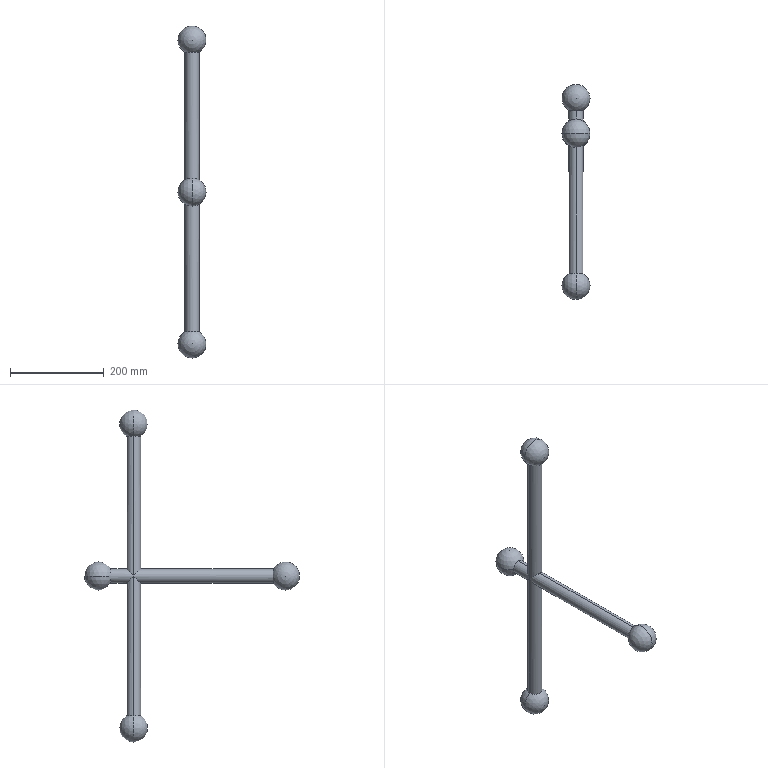Part | SolidWorks | features Revolution 3, ICE 2, Extrusion 1, MirrorPattern 1 | 1 solid | 16 faces | box 60 x 460 x 710 mm | volume 1097313 mm3 | sphere 8 | cylinder 8 | commonest cylinder face diameters 30 x8
STEP:
#1=CARTESIAN_POINT('',(0.,-355.,0.));
#2=VERTEX_POINT('',#1);
#3=CARTESIAN_POINT('',(0.,-299.019,-15.));
#4=VERTEX_POINT('',#3);
#5=CARTESIAN_POINT('',(0.,-325.,0.));
#6=DIRECTION('',(1.,0.,0.));
#7=DIRECTION('',(0.,0.,-1.));
#8=AXIS2_PLACEMENT_3D('',#5,#6,#7);
#9=CIRCLE('',#8,30.);
#10=EDGE_CURVE('',#2,#4,#9,.T.);
#11=ORIENTED_EDGE('',*,*,#10,.F.);
#12=CARTESIAN_POINT('',(0.,-299.019,15.));
#13=VERTEX_POINT('',#12);
#14=CARTESIAN_POINT('',(0.,-325.,0.));
#15=DIRECTION('',(-1.,0.,0.));
#16=DIRECTION('',(0.,0.,1.));
#17=AXIS2_PLACEMENT_3D('',#14,#15,#16);
#18=CIRCLE('',#17,30.);
#19=EDGE_CURVE('',#2,#13,#18,.T.);
#20=ORIENTED_EDGE('',*,*,#19,.T.);
#21=CARTESIAN_POINT('',(0.,-299.019,0.));
#22=DIRECTION('',(0.,-1.,0.));
#23=DIRECTION('',(0.,0.,-1.));
#24=AXIS2_PLACEMENT_3D('',#21,#22,#23);
#25=CIRCLE('',#24,15.);
#26=EDGE_CURVE('',#13,#4,#25,.T.);
#27=ORIENTED_EDGE('',*,*,#26,.T.);
#28=EDGE_LOOP('',(#11,#20,#27));
#29=FACE_OUTER_BOUND('',#28,.T.);
#30=CARTESIAN_POINT('',(0.,-325.,0.));
#31=DIRECTION('',(-1.,0.,0.));
#32=DIRECTION('',(0.,0.,-1.));
#33=AXIS2_PLACEMENT_3D('',#30,#31,#32);
#34=SPHERICAL_SURFACE('',#33,30.);
#35=ADVANCED_FACE('',(#29),#34,.T.);
#36=CARTESIAN_POINT('',(0.,-299.019,0.));
#37=DIRECTION('',(0.,-1.,0.));
#38=DIRECTION('',(0.,0.,-1.));
#39=AXIS2_PLACEMENT_3D('',#36,#37,#38);
#40=CIRCLE('',#39,15.);
#41=EDGE_CURVE('',#4,#13,#40,.T.);
#42=ORIENTED_EDGE('',*,*,#41,.F.);
#43=CARTESIAN_POINT('',(0.,-15.,-15.));
#44=VERTEX_POINT('',#43);
#45=CARTESIAN_POINT('',(0.,-300.,-15.));
#46=DIRECTION('',(0.,1.,0.));
#47=VECTOR('',#46,1000.);
#48=LINE('',#45,#47);
#49=EDGE_CURVE('',#4,#44,#48,.T.);
#50=ORIENTED_EDGE('',*,*,#49,.T.);
#51=CARTESIAN_POINT('',(15.,0.,0.));
#52=VERTEX_POINT('',#51);
#53=CARTESIAN_POINT('',(15.,0.,0.));
#54=CARTESIAN_POINT('',(15.,-8.787,-8.787));
#55=CARTESIAN_POINT('',(8.787,-15.,-15.));
#56=CARTESIAN_POINT('',(0.,-15.,-15.));
#57=(BOUNDED_CURVE()B_SPLINE_CURVE(3,(#53,#54,#55,#56),.UNSPECIFIED.,.F.,.T.)B_SPLINE_CURVE_WITH_KNOTS((4,4),(4.712,6.283),.UNSPECIFIED.)CURVE()GEOMETRIC_REPRESENTATION_ITEM()RATIONAL_B_SPLINE_CURVE((1.,0.8047,0.8047,1.))REPRESENTATION_ITEM(''));
#58=EDGE_CURVE('',#52,#44,#57,.T.);
#59=ORIENTED_EDGE('',*,*,#58,.F.);
#60=CARTESIAN_POINT('',(0.,-15.,15.));
#61=VERTEX_POINT('',#60);
#62=CARTESIAN_POINT('',(0.,-15.,15.));
#63=CARTESIAN_POINT('',(8.787,-15.,15.));
#64=CARTESIAN_POINT('',(15.,-8.787,8.787));
#65=CARTESIAN_POINT('',(15.,0.,0.));
#66=(BOUNDED_CURVE()B_SPLINE_CURVE(3,(#62,#63,#64,#65),.UNSPECIFIED.,.F.,.F.)B_SPLINE_CURVE_WITH_KNOTS((4,4),(3.142,4.712),.UNSPECIFIED.)CURVE()GEOMETRIC_REPRESENTATION_ITEM()RATIONAL_B_SPLINE_CURVE((1.,0.8047,0.8047,1.))REPRESENTATION_ITEM(''));
#67=EDGE_CURVE('',#61,#52,#66,.T.);
#68=ORIENTED_EDGE('',*,*,#67,.F.);
#69=CARTESIAN_POINT('',(0.,-300.,15.));
#70=DIRECTION('',(0.,1.,0.));
#71=VECTOR('',#70,1000.);
#72=LINE('',#69,#71);
#73=EDGE_CURVE('',#13,#61,#72,.T.);
#74=ORIENTED_EDGE('',*,*,#73,.F.);
#75=EDGE_LOOP('',(#42,#50,#59,#68,#74));
#76=FACE_OUTER_BOUND('',#75,.T.);
#77=CARTESIAN_POINT('',(0.,-300.,0.));
#78=DIRECTION('',(0.,1.,0.));
#79=DIRECTION('',(0.,0.,1.));
#80=AXIS2_PLACEMENT_3D('',#77,#78,#79);
#81=CYLINDRICAL_SURFACE('',#80,15.);
#82=ADVANCED_FACE('',(#76),#81,.T.);
#83=CARTESIAN_POINT('',(0.,49.019,-15.));
#84=VERTEX_POINT('',#83);
#85=CARTESIAN_POINT('',(-15.,49.019,0.));
#86=VERTEX_POINT('',#85);
#87=CARTESIAN_POINT('',(0.,49.019,0.));
#88=DIRECTION('',(0.,1.,0.));
#89=DIRECTION('',(0.,0.,1.));
#90=AXIS2_PLACEMENT_3D('',#87,#88,#89);
#91=CIRCLE('',#90,15.);
#92=EDGE_CURVE('',#84,#86,#91,.T.);
#93=ORIENTED_EDGE('',*,*,#92,.T.);
#94=CARTESIAN_POINT('',(0.,105.,0.));
#95=VERTEX_POINT('',#94);
#96=CARTESIAN_POINT('',(0.,75.,0.));
#97=DIRECTION('',(0.,0.,-1.));
#98=DIRECTION('',(-1.,0.,0.));
#99=AXIS2_PLACEMENT_3D('',#96,#97,#98);
#100=CIRCLE('',#99,30.);
#101=EDGE_CURVE('',#86,#95,#100,.T.);
#102=ORIENTED_EDGE('',*,*,#101,.T.);
#103=CARTESIAN_POINT('',(15.,49.019,0.));
#104=VERTEX_POINT('',#103);
#105=CARTESIAN_POINT('',(0.,75.,0.));
#106=DIRECTION('',(0.,0.,1.));
#107=DIRECTION('',(1.,0.,0.));
#108=AXIS2_PLACEMENT_3D('',#105,#106,#107);
#109=CIRCLE('',#108,30.);
#110=EDGE_CURVE('',#104,#95,#109,.T.);
#111=ORIENTED_EDGE('',*,*,#110,.F.);
#112=CARTESIAN_POINT('',(0.,49.019,0.));
#113=DIRECTION('',(0.,1.,0.));
#114=DIRECTION('',(0.,0.,1.));
#115=AXIS2_PLACEMENT_3D('',#112,#113,#114);
#116=CIRCLE('',#115,15.);
#117=EDGE_CURVE('',#104,#84,#116,.T.);
#118=ORIENTED_EDGE('',*,*,#117,.T.);
#119=EDGE_LOOP('',(#93,#102,#111,#118));
#120=FACE_OUTER_BOUND('',#119,.T.);
#121=CARTESIAN_POINT('',(0.,75.,0.));
#122=DIRECTION('',(0.,0.,-1.));
#123=DIRECTION('',(1.,0.,0.));
#124=AXIS2_PLACEMENT_3D('',#121,#122,#123);
#125=SPHERICAL_SURFACE('',#124,30.);
#126=ADVANCED_FACE('',(#120),#125,.T.);
#127=CARTESIAN_POINT('',(-15.,0.,299.019));
#128=VERTEX_POINT('',#127);
#129=CARTESIAN_POINT('',(15.,0.,299.019));
#130=VERTEX_POINT('',#129);
#131=CARTESIAN_POINT('',(0.,0.,299.019));
#132=DIRECTION('',(0.,0.,1.));
#133=DIRECTION('',(1.,0.,0.));
#134=AXIS2_PLACEMENT_3D('',#131,#132,#133);
#135=CIRCLE('',#134,15.);
#136=EDGE_CURVE('',#128,#130,#135,.T.);
#137=ORIENTED_EDGE('',*,*,#136,.T.);
#138=CARTESIAN_POINT('',(0.,0.,355.));
#139=VERTEX_POINT('',#138);
#140=CARTESIAN_POINT('',(0.,0.,325.));
#141=DIRECTION('',(0.,-1.,0.));
#142=DIRECTION('',(1.,0.,0.));
#143=AXIS2_PLACEMENT_3D('',#140,#141,#142);
#144=CIRCLE('',#143,30.);
#145=EDGE_CURVE('',#130,#139,#144,.T.);
#146=ORIENTED_EDGE('',*,*,#145,.T.);
#147=CARTESIAN_POINT('',(0.,0.,325.));
#148=DIRECTION('',(0.,1.,0.));
#149=DIRECTION('',(0.,0.,1.));
#150=AXIS2_PLACEMENT_3D('',#147,#148,#149);
#151=CIRCLE('',#150,30.);
#152=EDGE_CURVE('',#128,#139,#151,.T.);
#153=ORIENTED_EDGE('',*,*,#152,.F.);
#154=EDGE_LOOP('',(#137,#146,#153));
#155=FACE_OUTER_BOUND('',#154,.T.);
#156=CARTESIAN_POINT('',(0.,0.,325.));
#157=DIRECTION('',(0.,-1.,0.));
#158=DIRECTION('',(-1.,0.,0.));
#159=AXIS2_PLACEMENT_3D('',#156,#157,#158);
#160=SPHERICAL_SURFACE('',#159,30.);
#161=ADVANCED_FACE('',(#155),#160,.T.);
#162=CARTESIAN_POINT('',(-15.,0.,-299.019));
#163=VERTEX_POINT('',#162);
#164=CARTESIAN_POINT('',(15.,0.,-299.019));
#165=VERTEX_POINT('',#164);
#166=CARTESIAN_POINT('',(0.,0.,-299.019));
#167=DIRECTION('',(0.,0.,-1.));
#168=DIRECTION('',(-1.,0.,0.));
#169=AXIS2_PLACEMENT_3D('',#166,#167,#168);
#170=CIRCLE('',#169,15.);
#171=EDGE_CURVE('',#163,#165,#170,.T.);
#172=ORIENTED_EDGE('',*,*,#171,.T.);
#173=CARTESIAN_POINT('',(0.,0.,-355.));
#174=VERTEX_POINT('',#173);
#175=CARTESIAN_POINT('',(0.,0.,-325.));
#176=DIRECTION('',(0.,1.,0.));
#177=DIRECTION('',(-1.,0.,0.));
#178=AXIS2_PLACEMENT_3D('',#175,#176,#177);
#179=CIRCLE('',#178,30.);
#180=EDGE_CURVE('',#165,#174,#179,.T.);
#181=ORIENTED_EDGE('',*,*,#180,.T.);
#182=CARTESIAN_POINT('',(0.,0.,-325.));
#183=DIRECTION('',(0.,-1.,0.));
#184=DIRECTION('',(0.,0.,-1.));
#185=AXIS2_PLACEMENT_3D('',#182,#183,#184);
#186=CIRCLE('',#185,30.);
#187=EDGE_CURVE('',#163,#174,#186,.T.);
#188=ORIENTED_EDGE('',*,*,#187,.F.);
#189=EDGE_LOOP('',(#172,#181,#188));
#190=FACE_OUTER_BOUND('',#189,.T.);
#191=CARTESIAN_POINT('',(0.,0.,-325.));
#192=DIRECTION('',(0.,1.,0.));
#193=DIRECTION('',(-1.,0.,0.));
#194=AXIS2_PLACEMENT_3D('',#191,#192,#193);
#195=SPHERICAL_SURFACE('',#194,30.);
#196=ADVANCED_FACE('',(#190),#195,.T.);
#197=CARTESIAN_POINT('',(0.,0.,299.019));
#198=DIRECTION('',(0.,0.,1.));
#199=DIRECTION('',(1.,0.,0.));
#200=AXIS2_PLACEMENT_3D('',#197,#198,#199);
#201=CIRCLE('',#200,15.);
#202=EDGE_CURVE('',#130,#128,#201,.T.);
#203=ORIENTED_EDGE('',*,*,#202,.F.);
#204=CARTESIAN_POINT('',(15.,0.,300.));
#205=DIRECTION('',(0.,0.,-1.));
#206=VECTOR('',#205,1000.);
#207=LINE('',#204,#206);
#208=EDGE_CURVE('',#130,#52,#207,.T.);
#209=ORIENTED_EDGE('',*,*,#208,.T.);
#210=CARTESIAN_POINT('',(0.,15.,15.));
#211=VERTEX_POINT('',#210);
#212=CARTESIAN_POINT('',(0.,15.,15.));
#213=CARTESIAN_POINT('',(8.787,15.,15.));
#214=CARTESIAN_POINT('',(15.,8.787,8.787));
#215=CARTESIAN_POINT('',(15.,0.,0.));
#216=(BOUNDED_CURVE()B_SPLINE_CURVE(3,(#212,#213,#214,#215),.UNSPECIFIED.,.F.,.F.)B_SPLINE_CURVE_WITH_KNOTS((4,4),(3.142,4.712),.UNSPECIFIED.)CURVE()GEOMETRIC_REPRESENTATION_ITEM()RATIONAL_B_SPLINE_CURVE((1.,0.8047,0.8047,1.))REPRESENTATION_ITEM(''));
#217=EDGE_CURVE('',#211,#52,#216,.T.);
#218=ORIENTED_EDGE('',*,*,#217,.F.);
#219=CARTESIAN_POINT('',(-15.,0.,0.));
#220=VERTEX_POINT('',#219);
#221=CARTESIAN_POINT('',(-15.,0.,0.));
#222=CARTESIAN_POINT('',(-15.,8.787,8.787));
#223=CARTESIAN_POINT('',(-8.787,15.,15.));
#224=CARTESIAN_POINT('',(0.,15.,15.));
#225=(BOUNDED_CURVE()B_SPLINE_CURVE(3,(#221,#222,#223,#224),.UNSPECIFIED.,.F.,.F.)B_SPLINE_CURVE_WITH_KNOTS((4,4),(1.571,3.142),.UNSPECIFIED.)CURVE()GEOMETRIC_REPRESENTATION_ITEM()RATIONAL_B_SPLINE_CURVE((1.,0.8047,0.8047,1.))REPRESENTATION_ITEM(''));
#226=EDGE_CURVE('',#220,#211,#225,.T.);
#227=ORIENTED_EDGE('',*,*,#226,.F.);
#228=CARTESIAN_POINT('',(-15.,0.,300.));
#229=DIRECTION('',(0.,0.,-1.));
#230=VECTOR('',#229,1000.);
#231=LINE('',#228,#230);
#232=EDGE_CURVE('',#128,#220,#231,.T.);
#233=ORIENTED_EDGE('',*,*,#232,.F.);
#234=EDGE_LOOP('',(#203,#209,#218,#227,#233));
#235=FACE_OUTER_BOUND('',#234,.T.);
#236=CARTESIAN_POINT('',(0.,0.,300.));
#237=DIRECTION('',(0.,0.,-1.));
#238=DIRECTION('',(-1.,0.,0.));
#239=AXIS2_PLACEMENT_3D('',#236,#237,#238);
#240=CYLINDRICAL_SURFACE('',#239,15.);
#241=ADVANCED_FACE('',(#235),#240,.T.);
#242=CARTESIAN_POINT('',(0.,49.019,15.));
#243=VERTEX_POINT('',#242);
#244=CARTESIAN_POINT('',(0.,49.019,0.));
#245=DIRECTION('',(0.,1.,0.));
#246=DIRECTION('',(0.,0.,1.));
#247=AXIS2_PLACEMENT_3D('',#244,#245,#246);
#248=CIRCLE('',#247,15.);
#249=EDGE_CURVE('',#243,#104,#248,.T.);
#250=ORIENTED_EDGE('',*,*,#249,.F.);
#251=CARTESIAN_POINT('',(0.,50.,15.));
#252=DIRECTION('',(0.,-1.,0.));
#253=VECTOR('',#252,1000.);
#254=LINE('',#251,#253);
#255=EDGE_CURVE('',#243,#211,#254,.T.);
#256=ORIENTED_EDGE('',*,*,#255,.T.);
#257=ORIENTED_EDGE('',*,*,#217,.T.);
#258=CARTESIAN_POINT('',(0.,15.,-15.));
#259=VERTEX_POINT('',#258);
#260=CARTESIAN_POINT('',(15.,0.,0.));
#261=CARTESIAN_POINT('',(15.,8.787,-8.787));
#262=CARTESIAN_POINT('',(8.787,15.,-15.));
#263=CARTESIAN_POINT('',(0.,15.,-15.));
#264=(BOUNDED_CURVE()B_SPLINE_CURVE(3,(#260,#261,#262,#263),.UNSPECIFIED.,.F.,.F.)B_SPLINE_CURVE_WITH_KNOTS((4,4),(4.712,6.283),.UNSPECIFIED.)CURVE()GEOMETRIC_REPRESENTATION_ITEM()RATIONAL_B_SPLINE_CURVE((1.,0.8047,0.8047,1.))REPRESENTATION_ITEM(''));
#265=EDGE_CURVE('',#52,#259,#264,.T.);
#266=ORIENTED_EDGE('',*,*,#265,.T.);
#267=CARTESIAN_POINT('',(0.,50.,-15.));
#268=DIRECTION('',(0.,-1.,0.));
#269=VECTOR('',#268,1000.);
#270=LINE('',#267,#269);
#271=EDGE_CURVE('',#84,#259,#270,.T.);
#272=ORIENTED_EDGE('',*,*,#271,.F.);
#273=ORIENTED_EDGE('',*,*,#117,.F.);
#274=EDGE_LOOP('',(#250,#256,#257,#266,#272,#273));
#275=FACE_OUTER_BOUND('',#274,.T.);
#276=CARTESIAN_POINT('',(0.,50.,0.));
#277=DIRECTION('',(0.,-1.,0.));
#278=DIRECTION('',(0.,0.,-1.));
#279=AXIS2_PLACEMENT_3D('',#276,#277,#278);
#280=CYLINDRICAL_SURFACE('',#279,15.);
#281=ADVANCED_FACE('',(#275),#280,.T.);
#282=ORIENTED_EDGE('',*,*,#265,.F.);
#283=CARTESIAN_POINT('',(15.,0.,300.));
#284=DIRECTION('',(0.,0.,-1.));
#285=VECTOR('',#284,1000.);
#286=LINE('',#283,#285);
#287=EDGE_CURVE('',#52,#165,#286,.T.);
#288=ORIENTED_EDGE('',*,*,#287,.T.);
#289=ORIENTED_EDGE('',*,*,#171,.F.);
#290=CARTESIAN_POINT('',(-15.,0.,300.));
#291=DIRECTION('',(0.,0.,-1.));
#292=VECTOR('',#291,1000.);
#293=LINE('',#290,#292);
#294=EDGE_CURVE('',#220,#163,#293,.T.);
#295=ORIENTED_EDGE('',*,*,#294,.F.);
#296=CARTESIAN_POINT('',(0.,15.,-15.));
#297=CARTESIAN_POINT('',(-8.787,15.,-15.));
#298=CARTESIAN_POINT('',(-15.,8.787,-8.787));
#299=CARTESIAN_POINT('',(-15.,0.,0.));
#300=(BOUNDED_CURVE()B_SPLINE_CURVE(3,(#296,#297,#298,#299),.UNSPECIFIED.,.F.,.T.)B_SPLINE_CURVE_WITH_KNOTS((4,4),(0.,1.571),.UNSPECIFIED.)CURVE()GEOMETRIC_REPRESENTATION_ITEM()RATIONAL_B_SPLINE_CURVE((1.,0.8047,0.8047,1.))REPRESENTATION_ITEM(''));
#301=EDGE_CURVE('',#259,#220,#300,.T.);
#302=ORIENTED_EDGE('',*,*,#301,.F.);
#303=EDGE_LOOP('',(#282,#288,#289,#295,#302));
#304=FACE_OUTER_BOUND('',#303,.T.);
#305=CARTESIAN_POINT('',(0.,0.,300.));
#306=DIRECTION('',(0.,0.,-1.));
#307=DIRECTION('',(-1.,0.,0.));
#308=AXIS2_PLACEMENT_3D('',#305,#306,#307);
#309=CYLINDRICAL_SURFACE('',#308,15.);
#310=ADVANCED_FACE('',(#304),#309,.T.);
#311=ORIENTED_EDGE('',*,*,#287,.F.);
#312=ORIENTED_EDGE('',*,*,#58,.T.);
#313=CARTESIAN_POINT('',(0.,-15.,-15.));
#314=CARTESIAN_POINT('',(-8.787,-15.,-15.));
#315=CARTESIAN_POINT('',(-15.,-8.787,-8.787));
#316=CARTESIAN_POINT('',(-15.,0.,0.));
#317=(BOUNDED_CURVE()B_SPLINE_CURVE(3,(#313,#314,#315,#316),.UNSPECIFIED.,.F.,.F.)B_SPLINE_CURVE_WITH_KNOTS((4,4),(0.,1.571),.UNSPECIFIED.)CURVE()GEOMETRIC_REPRESENTATION_ITEM()RATIONAL_B_SPLINE_CURVE((1.,0.8047,0.8047,1.))REPRESENTATION_ITEM(''));
#318=EDGE_CURVE('',#44,#220,#317,.T.);
#319=ORIENTED_EDGE('',*,*,#318,.T.);
#320=ORIENTED_EDGE('',*,*,#294,.T.);
#321=CARTESIAN_POINT('',(0.,0.,-299.019));
#322=DIRECTION('',(0.,0.,-1.));
#323=DIRECTION('',(-1.,0.,0.));
#324=AXIS2_PLACEMENT_3D('',#321,#322,#323);
#325=CIRCLE('',#324,15.);
#326=EDGE_CURVE('',#165,#163,#325,.T.);
#327=ORIENTED_EDGE('',*,*,#326,.F.);
#328=EDGE_LOOP('',(#311,#312,#319,#320,#327));
#329=FACE_OUTER_BOUND('',#328,.T.);
#330=CARTESIAN_POINT('',(0.,0.,300.));
#331=DIRECTION('',(0.,0.,-1.));
#332=DIRECTION('',(-1.,0.,0.));
#333=AXIS2_PLACEMENT_3D('',#330,#331,#332);
#334=CYLINDRICAL_SURFACE('',#333,15.);
#335=ADVANCED_FACE('',(#329),#334,.T.);
#336=ORIENTED_EDGE('',*,*,#255,.F.);
#337=CARTESIAN_POINT('',(0.,49.019,0.));
#338=DIRECTION('',(0.,1.,0.));
#339=DIRECTION('',(0.,0.,1.));
#340=AXIS2_PLACEMENT_3D('',#337,#338,#339);
#341=CIRCLE('',#340,15.);
#342=EDGE_CURVE('',#86,#243,#341,.T.);
#343=ORIENTED_EDGE('',*,*,#342,.F.);
#344=ORIENTED_EDGE('',*,*,#92,.F.);
#345=ORIENTED_EDGE('',*,*,#271,.T.);
#346=ORIENTED_EDGE('',*,*,#301,.T.);
#347=ORIENTED_EDGE('',*,*,#226,.T.);
#348=EDGE_LOOP('',(#336,#343,#344,#345,#346,#347));
#349=FACE_OUTER_BOUND('',#348,.T.);
#350=CARTESIAN_POINT('',(0.,50.,0.));
#351=DIRECTION('',(0.,-1.,0.));
#352=DIRECTION('',(0.,0.,-1.));
#353=AXIS2_PLACEMENT_3D('',#350,#351,#352);
#354=CYLINDRICAL_SURFACE('',#353,15.);
#355=ADVANCED_FACE('',(#349),#354,.T.);
#356=ORIENTED_EDGE('',*,*,#208,.F.);
#357=ORIENTED_EDGE('',*,*,#136,.F.);
#358=ORIENTED_EDGE('',*,*,#232,.T.);
#359=CARTESIAN_POINT('',(-15.,0.,0.));
#360=CARTESIAN_POINT('',(-15.,-8.787,8.787));
#361=CARTESIAN_POINT('',(-8.787,-15.,15.));
#362=CARTESIAN_POINT('',(0.,-15.,15.));
#363=(BOUNDED_CURVE()B_SPLINE_CURVE(3,(#359,#360,#361,#362),.UNSPECIFIED.,.F.,.F.)B_SPLINE_CURVE_WITH_KNOTS((4,4),(1.571,3.142),.UNSPECIFIED.)CURVE()GEOMETRIC_REPRESENTATION_ITEM()RATIONAL_B_SPLINE_CURVE((1.,0.8047,0.8047,1.))REPRESENTATION_ITEM(''));
#364=EDGE_CURVE('',#220,#61,#363,.T.);
#365=ORIENTED_EDGE('',*,*,#364,.T.);
#366=ORIENTED_EDGE('',*,*,#67,.T.);
#367=EDGE_LOOP('',(#356,#357,#358,#365,#366));
#368=FACE_OUTER_BOUND('',#367,.T.);
#369=CARTESIAN_POINT('',(0.,0.,300.));
#370=DIRECTION('',(0.,0.,-1.));
#371=DIRECTION('',(-1.,0.,0.));
#372=AXIS2_PLACEMENT_3D('',#369,#370,#371);
#373=CYLINDRICAL_SURFACE('',#372,15.);
#374=ADVANCED_FACE('',(#368),#373,.T.);
#375=ORIENTED_EDGE('',*,*,#180,.F.);
#376=ORIENTED_EDGE('',*,*,#326,.T.);
#377=ORIENTED_EDGE('',*,*,#187,.T.);
#378=EDGE_LOOP('',(#375,#376,#377));
#379=FACE_OUTER_BOUND('',#378,.T.);
#380=CARTESIAN_POINT('',(0.,0.,-325.));
#381=DIRECTION('',(0.,1.,0.));
#382=DIRECTION('',(-1.,0.,0.));
#383=AXIS2_PLACEMENT_3D('',#380,#381,#382);
#384=SPHERICAL_SURFACE('',#383,30.);
#385=ADVANCED_FACE('',(#379),#384,.T.);
#386=ORIENTED_EDGE('',*,*,#145,.F.);
#387=ORIENTED_EDGE('',*,*,#202,.T.);
#388=ORIENTED_EDGE('',*,*,#152,.T.);
#389=EDGE_LOOP('',(#386,#387,#388));
#390=FACE_OUTER_BOUND('',#389,.T.);
#391=CARTESIAN_POINT('',(0.,0.,325.));
#392=DIRECTION('',(0.,-1.,0.));
#393=DIRECTION('',(-1.,0.,0.));
#394=AXIS2_PLACEMENT_3D('',#391,#392,#393);
#395=SPHERICAL_SURFACE('',#394,30.);
#396=ADVANCED_FACE('',(#390),#395,.T.);
#397=ORIENTED_EDGE('',*,*,#101,.F.);
#398=ORIENTED_EDGE('',*,*,#342,.T.);
#399=ORIENTED_EDGE('',*,*,#249,.T.);
#400=ORIENTED_EDGE('',*,*,#110,.T.);
#401=EDGE_LOOP('',(#397,#398,#399,#400));
#402=FACE_OUTER_BOUND('',#401,.T.);
#403=CARTESIAN_POINT('',(0.,75.,0.));
#404=DIRECTION('',(0.,0.,-1.));
#405=DIRECTION('',(1.,0.,0.));
#406=AXIS2_PLACEMENT_3D('',#403,#404,#405);
#407=SPHERICAL_SURFACE('',#406,30.);
#408=ADVANCED_FACE('',(#402),#407,.T.);
#409=ORIENTED_EDGE('',*,*,#49,.F.);
#410=ORIENTED_EDGE('',*,*,#26,.F.);
#411=ORIENTED_EDGE('',*,*,#73,.T.);
#412=ORIENTED_EDGE('',*,*,#364,.F.);
#413=ORIENTED_EDGE('',*,*,#318,.F.);
#414=EDGE_LOOP('',(#409,#410,#411,#412,#413));
#415=FACE_OUTER_BOUND('',#414,.T.);
#416=CARTESIAN_POINT('',(0.,-300.,0.));
#417=DIRECTION('',(0.,1.,0.));
#418=DIRECTION('',(0.,0.,1.));
#419=AXIS2_PLACEMENT_3D('',#416,#417,#418);
#420=CYLINDRICAL_SURFACE('',#419,15.);
#421=ADVANCED_FACE('',(#415),#420,.T.);
#422=ORIENTED_EDGE('',*,*,#19,.F.);
#423=ORIENTED_EDGE('',*,*,#10,.T.);
#424=ORIENTED_EDGE('',*,*,#41,.T.);
#425=EDGE_LOOP('',(#422,#423,#424));
#426=FACE_OUTER_BOUND('',#425,.T.);
#427=CARTESIAN_POINT('',(0.,-325.,0.));
#428=DIRECTION('',(-1.,0.,0.));
#429=DIRECTION('',(0.,0.,-1.));
#430=AXIS2_PLACEMENT_3D('',#427,#428,#429);
#431=SPHERICAL_SURFACE('',#430,30.);
#432=ADVANCED_FACE('',(#426),#431,.T.);
#433=CLOSED_SHELL('',(#35,#82,#126,#161,#196,#241,#281,#310,#335,#355,#374,#385,#396,#408,#421,#432));
#434=MANIFOLD_SOLID_BREP('',#433);
#435=CARTESIAN_POINT('',(0.,0.,0.));
#436=DIRECTION('',(0.,0.,1.));
#437=DIRECTION('',(1.,0.,0.));
#438=AXIS2_PLACEMENT_3D('',#435,#436,#437);
#439=(LENGTH_UNIT()NAMED_UNIT(*)SI_UNIT(.MILLI.,.METRE.));
#440=UNCERTAINTY_MEASURE_WITH_UNIT(LENGTH_MEASURE(0.00001),#439,'','');
#441=(NAMED_UNIT(*)PLANE_ANGLE_UNIT()SI_UNIT($,.RADIAN.));
#442=(NAMED_UNIT(*)SI_UNIT($,.STERADIAN.)SOLID_ANGLE_UNIT());
#443=(GEOMETRIC_REPRESENTATION_CONTEXT(3)GLOBAL_UNCERTAINTY_ASSIGNED_CONTEXT((#440))GLOBAL_UNIT_ASSIGNED_CONTEXT((#439,#441,#442))REPRESENTATION_CONTEXT('',''));
#444=ADVANCED_BREP_SHAPE_REPRESENTATION('',(#434,#438),#443);